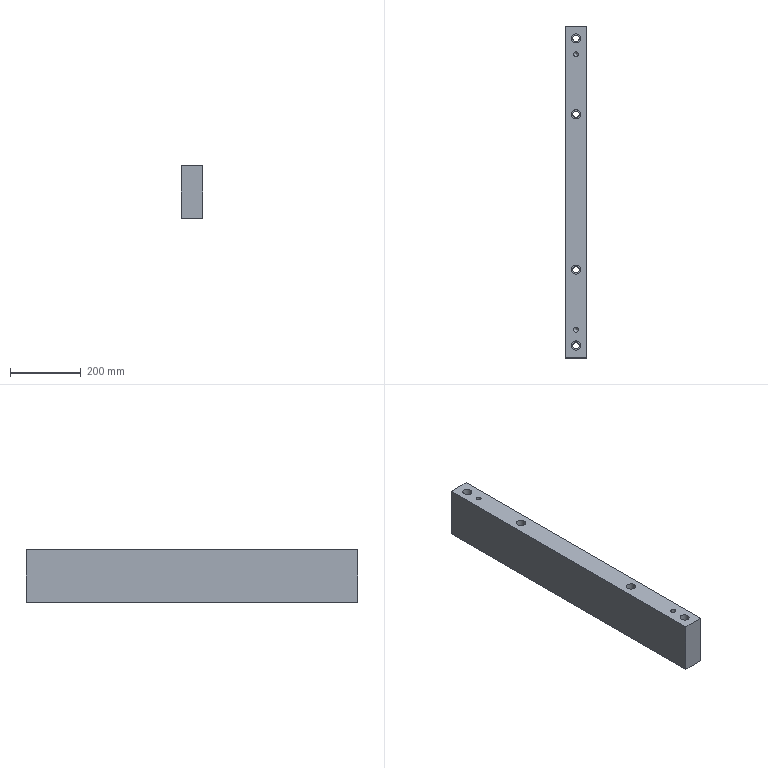Part | STEP file | lll_id1778_x_t | 1 solid | 22 faces | box 60 x 940 x 147.5 mm | volume 8080772 mm3 | plane 10 | cylinder 10 | cone 2 | commonest cylinder face diameters 18.009 x4 26.008 x4 14.506 x2
STEP:
#1=CARTESIAN_POINT('',(3486.439,220.,370.));
#2=VERTEX_POINT('',#1);
#3=CARTESIAN_POINT('',(3473.435,220.,370.));
#4=DIRECTION('',(0.,0.,1.));
#5=DIRECTION('',(1.,0.,0.));
#6=AXIS2_PLACEMENT_3D('',#3,#4,#5);
#7=CIRCLE('',#6,13.004);
#8=EDGE_CURVE('',#2,#2,#7,.T.);
#9=ORIENTED_EDGE('',*,*,#8,.F.);
#10=EDGE_LOOP('',(#9));
#11=FACE_BOUND('',#10,.T.);
#12=CARTESIAN_POINT('',(3486.439,-220.,370.));
#13=VERTEX_POINT('',#12);
#14=CARTESIAN_POINT('',(3473.435,-220.,370.));
#15=DIRECTION('',(0.,0.,-1.));
#16=DIRECTION('',(1.,0.,0.));
#17=AXIS2_PLACEMENT_3D('',#14,#15,#16);
#18=CIRCLE('',#17,13.004);
#19=EDGE_CURVE('',#13,#13,#18,.T.);
#20=ORIENTED_EDGE('',*,*,#19,.T.);
#21=EDGE_LOOP('',(#20));
#22=FACE_BOUND('',#21,.T.);
#23=CARTESIAN_POINT('',(3486.439,-435.,370.));
#24=VERTEX_POINT('',#23);
#25=CARTESIAN_POINT('',(3473.435,-435.,370.));
#26=DIRECTION('',(0.,0.,-1.));
#27=DIRECTION('',(1.,0.,0.));
#28=AXIS2_PLACEMENT_3D('',#25,#26,#27);
#29=CIRCLE('',#28,13.004);
#30=EDGE_CURVE('',#24,#24,#29,.T.);
#31=ORIENTED_EDGE('',*,*,#30,.T.);
#32=EDGE_LOOP('',(#31));
#33=FACE_BOUND('',#32,.T.);
#34=CARTESIAN_POINT('',(3503.435,470.,370.));
#35=VERTEX_POINT('',#34);
#36=CARTESIAN_POINT('',(3443.435,470.,370.));
#37=VERTEX_POINT('',#36);
#38=CARTESIAN_POINT('',(7413.435,470.,370.));
#39=DIRECTION('',(-1.,0.,0.));
#40=VECTOR('',#39,1.);
#41=LINE('',#38,#40);
#42=EDGE_CURVE('',#35,#37,#41,.T.);
#43=ORIENTED_EDGE('',*,*,#42,.T.);
#44=CARTESIAN_POINT('',(3443.435,-470.,370.));
#45=VERTEX_POINT('',#44);
#46=CARTESIAN_POINT('',(3443.435,600.,370.));
#47=DIRECTION('',(0.,-1.,0.));
#48=VECTOR('',#47,1.);
#49=LINE('',#46,#48);
#50=EDGE_CURVE('',#37,#45,#49,.T.);
#51=ORIENTED_EDGE('',*,*,#50,.T.);
#52=CARTESIAN_POINT('',(3503.435,-470.,370.));
#53=VERTEX_POINT('',#52);
#54=CARTESIAN_POINT('',(3443.435,-470.,370.));
#55=DIRECTION('',(1.,0.,0.));
#56=VECTOR('',#55,1.);
#57=LINE('',#54,#56);
#58=EDGE_CURVE('',#45,#53,#57,.T.);
#59=ORIENTED_EDGE('',*,*,#58,.T.);
#60=CARTESIAN_POINT('',(3503.435,1.,370.));
#61=DIRECTION('',(0.,1.,0.));
#62=VECTOR('',#61,1.);
#63=LINE('',#60,#62);
#64=EDGE_CURVE('',#53,#35,#63,.T.);
#65=ORIENTED_EDGE('',*,*,#64,.T.);
#66=EDGE_LOOP('',(#43,#51,#59,#65));
#67=FACE_BOUND('',#66,.T.);
#68=CARTESIAN_POINT('',(3486.439,435.,370.));
#69=VERTEX_POINT('',#68);
#70=CARTESIAN_POINT('',(3473.435,435.,370.));
#71=DIRECTION('',(0.,0.,1.));
#72=DIRECTION('',(1.,0.,0.));
#73=AXIS2_PLACEMENT_3D('',#70,#71,#72);
#74=CIRCLE('',#73,13.004);
#75=EDGE_CURVE('',#69,#69,#74,.T.);
#76=ORIENTED_EDGE('',*,*,#75,.F.);
#77=EDGE_LOOP('',(#76));
#78=FACE_BOUND('',#77,.T.);
#79=CARTESIAN_POINT('',(3480.688,-390.,370.));
#80=VERTEX_POINT('',#79);
#81=CARTESIAN_POINT('',(3473.435,-390.,370.));
#82=DIRECTION('',(0.,0.,-1.));
#83=DIRECTION('',(1.,0.,0.));
#84=AXIS2_PLACEMENT_3D('',#81,#82,#83);
#85=CIRCLE('',#84,7.253);
#86=EDGE_CURVE('',#80,#80,#85,.T.);
#87=ORIENTED_EDGE('',*,*,#86,.T.);
#88=EDGE_LOOP('',(#87));
#89=FACE_BOUND('',#88,.T.);
#90=CARTESIAN_POINT('',(3480.688,390.,370.));
#91=VERTEX_POINT('',#90);
#92=CARTESIAN_POINT('',(3473.435,390.,370.));
#93=DIRECTION('',(0.,0.,1.));
#94=DIRECTION('',(1.,0.,0.));
#95=AXIS2_PLACEMENT_3D('',#92,#93,#94);
#96=CIRCLE('',#95,7.253);
#97=EDGE_CURVE('',#91,#91,#96,.T.);
#98=ORIENTED_EDGE('',*,*,#97,.F.);
#99=EDGE_LOOP('',(#98));
#100=FACE_BOUND('',#99,.T.);
#101=CARTESIAN_POINT('',(1257.12,1.,370.));
#102=DIRECTION('',(0.,0.,-1.));
#103=DIRECTION('',(1.,0.,0.));
#104=AXIS2_PLACEMENT_3D('',#101,#102,#103);
#105=PLANE('',#104);
#106=ADVANCED_FACE('',(#11,#22,#33,#67,#78,#89,#100),#105,.F.);
#107=CARTESIAN_POINT('',(3482.44,435.,222.5));
#108=VERTEX_POINT('',#107);
#109=CARTESIAN_POINT('',(3473.435,435.,222.5));
#110=DIRECTION('',(0.,0.,-1.));
#111=DIRECTION('',(1.,0.,0.));
#112=AXIS2_PLACEMENT_3D('',#109,#110,#111);
#113=CIRCLE('',#112,9.005);
#114=EDGE_CURVE('',#108,#108,#113,.T.);
#115=ORIENTED_EDGE('',*,*,#114,.F.);
#116=EDGE_LOOP('',(#115));
#117=FACE_BOUND('',#116,.T.);
#118=CARTESIAN_POINT('',(3482.44,220.,222.5));
#119=VERTEX_POINT('',#118);
#120=CARTESIAN_POINT('',(3473.435,220.,222.5));
#121=DIRECTION('',(0.,0.,-1.));
#122=DIRECTION('',(1.,0.,0.));
#123=AXIS2_PLACEMENT_3D('',#120,#121,#122);
#124=CIRCLE('',#123,9.005);
#125=EDGE_CURVE('',#119,#119,#124,.T.);
#126=ORIENTED_EDGE('',*,*,#125,.F.);
#127=EDGE_LOOP('',(#126));
#128=FACE_BOUND('',#127,.T.);
#129=CARTESIAN_POINT('',(3482.44,-435.,222.5));
#130=VERTEX_POINT('',#129);
#131=CARTESIAN_POINT('',(3473.435,-435.,222.5));
#132=DIRECTION('',(0.,0.,1.));
#133=DIRECTION('',(1.,0.,0.));
#134=AXIS2_PLACEMENT_3D('',#131,#132,#133);
#135=CIRCLE('',#134,9.005);
#136=EDGE_CURVE('',#130,#130,#135,.T.);
#137=ORIENTED_EDGE('',*,*,#136,.T.);
#138=EDGE_LOOP('',(#137));
#139=FACE_BOUND('',#138,.T.);
#140=CARTESIAN_POINT('',(3503.435,470.,222.5));
#141=VERTEX_POINT('',#140);
#142=CARTESIAN_POINT('',(3503.435,-470.,222.5));
#143=VERTEX_POINT('',#142);
#144=CARTESIAN_POINT('',(3503.435,1.,222.5));
#145=DIRECTION('',(0.,-1.,0.));
#146=VECTOR('',#145,1.);
#147=LINE('',#144,#146);
#148=EDGE_CURVE('',#141,#143,#147,.T.);
#149=ORIENTED_EDGE('',*,*,#148,.T.);
#150=CARTESIAN_POINT('',(3443.435,-470.,222.5));
#151=VERTEX_POINT('',#150);
#152=CARTESIAN_POINT('',(3443.435,-470.,222.5));
#153=DIRECTION('',(1.,0.,0.));
#154=VECTOR('',#153,1.);
#155=LINE('',#152,#154);
#156=EDGE_CURVE('',#151,#143,#155,.T.);
#157=ORIENTED_EDGE('',*,*,#156,.F.);
#158=CARTESIAN_POINT('',(3443.435,470.,222.5));
#159=VERTEX_POINT('',#158);
#160=CARTESIAN_POINT('',(3443.435,600.,222.5));
#161=DIRECTION('',(0.,-1.,0.));
#162=VECTOR('',#161,1.);
#163=LINE('',#160,#162);
#164=EDGE_CURVE('',#159,#151,#163,.T.);
#165=ORIENTED_EDGE('',*,*,#164,.F.);
#166=CARTESIAN_POINT('',(7413.435,470.,222.5));
#167=DIRECTION('',(-1.,0.,0.));
#168=VECTOR('',#167,1.);
#169=LINE('',#166,#168);
#170=EDGE_CURVE('',#141,#159,#169,.T.);
#171=ORIENTED_EDGE('',*,*,#170,.F.);
#172=EDGE_LOOP('',(#149,#157,#165,#171));
#173=FACE_BOUND('',#172,.T.);
#174=CARTESIAN_POINT('',(3482.44,-220.,222.5));
#175=VERTEX_POINT('',#174);
#176=CARTESIAN_POINT('',(3473.435,-220.,222.5));
#177=DIRECTION('',(0.,0.,1.));
#178=DIRECTION('',(1.,0.,0.));
#179=AXIS2_PLACEMENT_3D('',#176,#177,#178);
#180=CIRCLE('',#179,9.005);
#181=EDGE_CURVE('',#175,#175,#180,.T.);
#182=ORIENTED_EDGE('',*,*,#181,.T.);
#183=EDGE_LOOP('',(#182));
#184=FACE_BOUND('',#183,.T.);
#185=CARTESIAN_POINT('',(1257.12,1.,222.5));
#186=DIRECTION('',(0.,0.,-1.));
#187=DIRECTION('',(1.,0.,0.));
#188=AXIS2_PLACEMENT_3D('',#185,#186,#187);
#189=PLANE('',#188);
#190=ADVANCED_FACE('',(#117,#128,#139,#173,#184),#189,.T.);
#191=ORIENTED_EDGE('',*,*,#164,.T.);
#192=CARTESIAN_POINT('',(3443.435,-470.,360.));
#193=DIRECTION('',(0.,0.,-1.));
#194=VECTOR('',#193,1.);
#195=LINE('',#192,#194);
#196=EDGE_CURVE('',#45,#151,#195,.T.);
#197=ORIENTED_EDGE('',*,*,#196,.F.);
#198=ORIENTED_EDGE('',*,*,#50,.F.);
#199=CARTESIAN_POINT('',(3443.435,470.,360.));
#200=DIRECTION('',(0.,0.,-1.));
#201=VECTOR('',#200,1.);
#202=LINE('',#199,#201);
#203=EDGE_CURVE('',#37,#159,#202,.T.);
#204=ORIENTED_EDGE('',*,*,#203,.T.);
#205=EDGE_LOOP('',(#191,#197,#198,#204));
#206=FACE_OUTER_BOUND('',#205,.T.);
#207=CARTESIAN_POINT('',(3443.435,600.,360.));
#208=DIRECTION('',(-1.,0.,0.));
#209=DIRECTION('',(0.,0.,-1.));
#210=AXIS2_PLACEMENT_3D('',#207,#208,#209);
#211=PLANE('',#210);
#212=ADVANCED_FACE('',(#206),#211,.T.);
#213=CARTESIAN_POINT('',(3503.435,-470.,360.));
#214=DIRECTION('',(0.,0.,-1.));
#215=VECTOR('',#214,1.);
#216=LINE('',#213,#215);
#217=EDGE_CURVE('',#53,#143,#216,.T.);
#218=ORIENTED_EDGE('',*,*,#217,.F.);
#219=ORIENTED_EDGE('',*,*,#58,.F.);
#220=ORIENTED_EDGE('',*,*,#196,.T.);
#221=ORIENTED_EDGE('',*,*,#156,.T.);
#222=EDGE_LOOP('',(#218,#219,#220,#221));
#223=FACE_OUTER_BOUND('',#222,.T.);
#224=CARTESIAN_POINT('',(3443.435,-470.,360.));
#225=DIRECTION('',(0.,-1.,0.));
#226=DIRECTION('',(0.,0.,-1.));
#227=AXIS2_PLACEMENT_3D('',#224,#225,#226);
#228=PLANE('',#227);
#229=ADVANCED_FACE('',(#223),#228,.T.);
#230=CARTESIAN_POINT('',(3503.435,470.,360.));
#231=DIRECTION('',(0.,0.,1.));
#232=VECTOR('',#231,1.);
#233=LINE('',#230,#232);
#234=EDGE_CURVE('',#141,#35,#233,.T.);
#235=ORIENTED_EDGE('',*,*,#234,.F.);
#236=ORIENTED_EDGE('',*,*,#170,.T.);
#237=ORIENTED_EDGE('',*,*,#203,.F.);
#238=ORIENTED_EDGE('',*,*,#42,.F.);
#239=EDGE_LOOP('',(#235,#236,#237,#238));
#240=FACE_OUTER_BOUND('',#239,.T.);
#241=CARTESIAN_POINT('',(7413.435,470.,360.));
#242=DIRECTION('',(0.,1.,0.));
#243=DIRECTION('',(0.,0.,1.));
#244=AXIS2_PLACEMENT_3D('',#241,#242,#243);
#245=PLANE('',#244);
#246=ADVANCED_FACE('',(#240),#245,.T.);
#247=ORIENTED_EDGE('',*,*,#234,.T.);
#248=ORIENTED_EDGE('',*,*,#64,.F.);
#249=ORIENTED_EDGE('',*,*,#217,.T.);
#250=ORIENTED_EDGE('',*,*,#148,.F.);
#251=EDGE_LOOP('',(#247,#248,#249,#250));
#252=FACE_OUTER_BOUND('',#251,.T.);
#253=CARTESIAN_POINT('',(3503.435,0.,291.25));
#254=DIRECTION('',(-1.,0.,0.));
#255=DIRECTION('',(0.,0.,-1.));
#256=AXIS2_PLACEMENT_3D('',#253,#254,#255);
#257=PLANE('',#256);
#258=ADVANCED_FACE('',(#252),#257,.F.);
#259=CARTESIAN_POINT('',(3464.431,-435.,302.5));
#260=VERTEX_POINT('',#259);
#261=CARTESIAN_POINT('',(3473.435,-435.,302.5));
#262=DIRECTION('',(0.,0.,-1.));
#263=DIRECTION('',(-1.,0.,0.));
#264=AXIS2_PLACEMENT_3D('',#261,#262,#263);
#265=CIRCLE('',#264,9.005);
#266=EDGE_CURVE('',#260,#260,#265,.T.);
#267=ORIENTED_EDGE('',*,*,#266,.F.);
#268=EDGE_LOOP('',(#267));
#269=FACE_BOUND('',#268,.T.);
#270=ORIENTED_EDGE('',*,*,#136,.F.);
#271=EDGE_LOOP('',(#270));
#272=FACE_BOUND('',#271,.T.);
#273=CARTESIAN_POINT('',(3473.435,-435.,420.));
#274=DIRECTION('',(0.,0.,-1.));
#275=DIRECTION('',(1.,0.,0.));
#276=AXIS2_PLACEMENT_3D('',#273,#274,#275);
#277=CYLINDRICAL_SURFACE('',#276,9.005);
#278=ADVANCED_FACE('',(#269,#272),#277,.F.);
#279=ORIENTED_EDGE('',*,*,#266,.T.);
#280=EDGE_LOOP('',(#279));
#281=FACE_BOUND('',#280,.T.);
#282=CARTESIAN_POINT('',(3486.439,-435.,302.5));
#283=VERTEX_POINT('',#282);
#284=CARTESIAN_POINT('',(3473.435,-435.,302.5));
#285=DIRECTION('',(0.,0.,-1.));
#286=DIRECTION('',(-1.,0.,0.));
#287=AXIS2_PLACEMENT_3D('',#284,#285,#286);
#288=CIRCLE('',#287,13.004);
#289=EDGE_CURVE('',#283,#283,#288,.T.);
#290=ORIENTED_EDGE('',*,*,#289,.F.);
#291=EDGE_LOOP('',(#290));
#292=FACE_BOUND('',#291,.T.);
#293=CARTESIAN_POINT('',(3473.435,-435.,302.5));
#294=DIRECTION('',(0.,0.,-1.));
#295=DIRECTION('',(-1.,0.,0.));
#296=AXIS2_PLACEMENT_3D('',#293,#294,#295);
#297=PLANE('',#296);
#298=ADVANCED_FACE('',(#281,#292),#297,.F.);
#299=ORIENTED_EDGE('',*,*,#289,.T.);
#300=EDGE_LOOP('',(#299));
#301=FACE_BOUND('',#300,.T.);
#302=ORIENTED_EDGE('',*,*,#30,.F.);
#303=EDGE_LOOP('',(#302));
#304=FACE_BOUND('',#303,.T.);
#305=CARTESIAN_POINT('',(3473.435,-435.,420.));
#306=DIRECTION('',(0.,0.,-1.));
#307=DIRECTION('',(1.,0.,0.));
#308=AXIS2_PLACEMENT_3D('',#305,#306,#307);
#309=CYLINDRICAL_SURFACE('',#308,13.004);
#310=ADVANCED_FACE('',(#301,#304),#309,.F.);
#311=CARTESIAN_POINT('',(3464.431,-220.,302.5));
#312=VERTEX_POINT('',#311);
#313=CARTESIAN_POINT('',(3473.435,-220.,302.5));
#314=DIRECTION('',(0.,0.,-1.));
#315=DIRECTION('',(-1.,0.,0.));
#316=AXIS2_PLACEMENT_3D('',#313,#314,#315);
#317=CIRCLE('',#316,9.005);
#318=EDGE_CURVE('',#312,#312,#317,.T.);
#319=ORIENTED_EDGE('',*,*,#318,.F.);
#320=EDGE_LOOP('',(#319));
#321=FACE_BOUND('',#320,.T.);
#322=ORIENTED_EDGE('',*,*,#181,.F.);
#323=EDGE_LOOP('',(#322));
#324=FACE_BOUND('',#323,.T.);
#325=CARTESIAN_POINT('',(3473.435,-220.,420.));
#326=DIRECTION('',(0.,0.,-1.));
#327=DIRECTION('',(1.,0.,0.));
#328=AXIS2_PLACEMENT_3D('',#325,#326,#327);
#329=CYLINDRICAL_SURFACE('',#328,9.005);
#330=ADVANCED_FACE('',(#321,#324),#329,.F.);
#331=ORIENTED_EDGE('',*,*,#318,.T.);
#332=EDGE_LOOP('',(#331));
#333=FACE_BOUND('',#332,.T.);
#334=CARTESIAN_POINT('',(3486.439,-220.,302.5));
#335=VERTEX_POINT('',#334);
#336=CARTESIAN_POINT('',(3473.435,-220.,302.5));
#337=DIRECTION('',(0.,0.,-1.));
#338=DIRECTION('',(1.,0.,0.));
#339=AXIS2_PLACEMENT_3D('',#336,#337,#338);
#340=CIRCLE('',#339,13.004);
#341=EDGE_CURVE('',#335,#335,#340,.T.);
#342=ORIENTED_EDGE('',*,*,#341,.F.);
#343=EDGE_LOOP('',(#342));
#344=FACE_BOUND('',#343,.T.);
#345=CARTESIAN_POINT('',(3473.435,-220.,302.5));
#346=DIRECTION('',(0.,0.,-1.));
#347=DIRECTION('',(-1.,0.,0.));
#348=AXIS2_PLACEMENT_3D('',#345,#346,#347);
#349=PLANE('',#348);
#350=ADVANCED_FACE('',(#333,#344),#349,.F.);
#351=ORIENTED_EDGE('',*,*,#341,.T.);
#352=EDGE_LOOP('',(#351));
#353=FACE_BOUND('',#352,.T.);
#354=ORIENTED_EDGE('',*,*,#19,.F.);
#355=EDGE_LOOP('',(#354));
#356=FACE_BOUND('',#355,.T.);
#357=CARTESIAN_POINT('',(3473.435,-220.,420.));
#358=DIRECTION('',(0.,0.,-1.));
#359=DIRECTION('',(1.,0.,0.));
#360=AXIS2_PLACEMENT_3D('',#357,#358,#359);
#361=CYLINDRICAL_SURFACE('',#360,13.004);
#362=ADVANCED_FACE('',(#353,#356),#361,.F.);
#363=CARTESIAN_POINT('',(3464.431,220.,302.5));
#364=VERTEX_POINT('',#363);
#365=CARTESIAN_POINT('',(3473.435,220.,302.5));
#366=DIRECTION('',(0.,0.,1.));
#367=DIRECTION('',(-1.,0.,0.));
#368=AXIS2_PLACEMENT_3D('',#365,#366,#367);
#369=CIRCLE('',#368,9.005);
#370=EDGE_CURVE('',#364,#364,#369,.T.);
#371=ORIENTED_EDGE('',*,*,#370,.T.);
#372=EDGE_LOOP('',(#371));
#373=FACE_BOUND('',#372,.T.);
#374=ORIENTED_EDGE('',*,*,#125,.T.);
#375=EDGE_LOOP('',(#374));
#376=FACE_BOUND('',#375,.T.);
#377=CARTESIAN_POINT('',(3473.435,220.,420.));
#378=DIRECTION('',(0.,0.,-1.));
#379=DIRECTION('',(1.,0.,0.));
#380=AXIS2_PLACEMENT_3D('',#377,#378,#379);
#381=CYLINDRICAL_SURFACE('',#380,9.005);
#382=ADVANCED_FACE('',(#373,#376),#381,.F.);
#383=ORIENTED_EDGE('',*,*,#370,.F.);
#384=EDGE_LOOP('',(#383));
#385=FACE_BOUND('',#384,.T.);
#386=CARTESIAN_POINT('',(3486.439,220.,302.5));
#387=VERTEX_POINT('',#386);
#388=CARTESIAN_POINT('',(3473.435,220.,302.5));
#389=DIRECTION('',(0.,0.,1.));
#390=DIRECTION('',(1.,0.,0.));
#391=AXIS2_PLACEMENT_3D('',#388,#389,#390);
#392=CIRCLE('',#391,13.004);
#393=EDGE_CURVE('',#387,#387,#392,.T.);
#394=ORIENTED_EDGE('',*,*,#393,.T.);
#395=EDGE_LOOP('',(#394));
#396=FACE_BOUND('',#395,.T.);
#397=CARTESIAN_POINT('',(3473.435,220.,302.5));
#398=DIRECTION('',(0.,0.,-1.));
#399=DIRECTION('',(-1.,0.,0.));
#400=AXIS2_PLACEMENT_3D('',#397,#398,#399);
#401=PLANE('',#400);
#402=ADVANCED_FACE('',(#385,#396),#401,.F.);
#403=ORIENTED_EDGE('',*,*,#393,.F.);
#404=EDGE_LOOP('',(#403));
#405=FACE_BOUND('',#404,.T.);
#406=ORIENTED_EDGE('',*,*,#8,.T.);
#407=EDGE_LOOP('',(#406));
#408=FACE_BOUND('',#407,.T.);
#409=CARTESIAN_POINT('',(3473.435,220.,420.));
#410=DIRECTION('',(0.,0.,-1.));
#411=DIRECTION('',(1.,0.,0.));
#412=AXIS2_PLACEMENT_3D('',#409,#410,#411);
#413=CYLINDRICAL_SURFACE('',#412,13.004);
#414=ADVANCED_FACE('',(#405,#408),#413,.F.);
#415=CARTESIAN_POINT('',(3464.431,435.,302.5));
#416=VERTEX_POINT('',#415);
#417=CARTESIAN_POINT('',(3473.435,435.,302.5));
#418=DIRECTION('',(0.,0.,1.));
#419=DIRECTION('',(-1.,0.,0.));
#420=AXIS2_PLACEMENT_3D('',#417,#418,#419);
#421=CIRCLE('',#420,9.005);
#422=EDGE_CURVE('',#416,#416,#421,.T.);
#423=ORIENTED_EDGE('',*,*,#422,.T.);
#424=EDGE_LOOP('',(#423));
#425=FACE_BOUND('',#424,.T.);
#426=ORIENTED_EDGE('',*,*,#114,.T.);
#427=EDGE_LOOP('',(#426));
#428=FACE_BOUND('',#427,.T.);
#429=CARTESIAN_POINT('',(3473.435,435.,420.));
#430=DIRECTION('',(0.,0.,-1.));
#431=DIRECTION('',(1.,0.,0.));
#432=AXIS2_PLACEMENT_3D('',#429,#430,#431);
#433=CYLINDRICAL_SURFACE('',#432,9.005);
#434=ADVANCED_FACE('',(#425,#428),#433,.F.);
#435=ORIENTED_EDGE('',*,*,#422,.F.);
#436=EDGE_LOOP('',(#435));
#437=FACE_BOUND('',#436,.T.);
#438=CARTESIAN_POINT('',(3486.439,435.,302.5));
#439=VERTEX_POINT('',#438);
#440=CARTESIAN_POINT('',(3473.435,435.,302.5));
#441=DIRECTION('',(0.,0.,1.));
#442=DIRECTION('',(1.,0.,0.));
#443=AXIS2_PLACEMENT_3D('',#440,#441,#442);
#444=CIRCLE('',#443,13.004);
#445=EDGE_CURVE('',#439,#439,#444,.T.);
#446=ORIENTED_EDGE('',*,*,#445,.T.);
#447=EDGE_LOOP('',(#446));
#448=FACE_BOUND('',#447,.T.);
#449=CARTESIAN_POINT('',(3473.435,435.,302.5));
#450=DIRECTION('',(0.,0.,-1.));
#451=DIRECTION('',(-1.,0.,0.));
#452=AXIS2_PLACEMENT_3D('',#449,#450,#451);
#453=PLANE('',#452);
#454=ADVANCED_FACE('',(#437,#448),#453,.F.);
#455=ORIENTED_EDGE('',*,*,#445,.F.);
#456=EDGE_LOOP('',(#455));
#457=FACE_BOUND('',#456,.T.);
#458=ORIENTED_EDGE('',*,*,#75,.T.);
#459=EDGE_LOOP('',(#458));
#460=FACE_BOUND('',#459,.T.);
#461=CARTESIAN_POINT('',(3473.435,435.,420.));
#462=DIRECTION('',(0.,0.,-1.));
#463=DIRECTION('',(1.,0.,0.));
#464=AXIS2_PLACEMENT_3D('',#461,#462,#463);
#465=CYLINDRICAL_SURFACE('',#464,13.004);
#466=ADVANCED_FACE('',(#457,#460),#465,.F.);
#467=CARTESIAN_POINT('',(3466.182,-390.,332.247));
#468=VERTEX_POINT('',#467);
#469=CARTESIAN_POINT('',(3473.435,-390.,332.247));
#470=DIRECTION('',(0.,0.,-1.));
#471=DIRECTION('',(-1.,0.,0.));
#472=AXIS2_PLACEMENT_3D('',#469,#470,#471);
#473=CIRCLE('',#472,7.253);
#474=EDGE_CURVE('',#468,#468,#473,.T.);
#475=ORIENTED_EDGE('',*,*,#474,.T.);
#476=EDGE_LOOP('',(#475));
#477=FACE_BOUND('',#476,.T.);
#478=ORIENTED_EDGE('',*,*,#86,.F.);
#479=EDGE_LOOP('',(#478));
#480=FACE_BOUND('',#479,.T.);
#481=CARTESIAN_POINT('',(3473.435,-390.,370.));
#482=DIRECTION('',(0.,0.,-1.));
#483=DIRECTION('',(1.,0.,0.));
#484=AXIS2_PLACEMENT_3D('',#481,#482,#483);
#485=CYLINDRICAL_SURFACE('',#484,7.253);
#486=ADVANCED_FACE('',(#477,#480),#485,.F.);
#487=CARTESIAN_POINT('',(3473.435,-390.,324.994));
#488=VERTEX_POINT('',#487);
#489=VERTEX_LOOP('',#488);
#490=FACE_BOUND('',#489,.T.);
#491=ORIENTED_EDGE('',*,*,#474,.F.);
#492=EDGE_LOOP('',(#491));
#493=FACE_BOUND('',#492,.T.);
#494=CARTESIAN_POINT('',(3473.435,-390.,332.247));
#495=DIRECTION('',(0.,0.,1.));
#496=DIRECTION('',(1.,0.,0.));
#497=AXIS2_PLACEMENT_3D('',#494,#495,#496);
#498=CONICAL_SURFACE('',#497,7.253,45.);
#499=ADVANCED_FACE('',(#490,#493),#498,.F.);
#500=CARTESIAN_POINT('',(3466.182,390.,332.247));
#501=VERTEX_POINT('',#500);
#502=CARTESIAN_POINT('',(3473.435,390.,332.247));
#503=DIRECTION('',(0.,0.,1.));
#504=DIRECTION('',(-1.,0.,0.));
#505=AXIS2_PLACEMENT_3D('',#502,#503,#504);
#506=CIRCLE('',#505,7.253);
#507=EDGE_CURVE('',#501,#501,#506,.T.);
#508=ORIENTED_EDGE('',*,*,#507,.F.);
#509=EDGE_LOOP('',(#508));
#510=FACE_BOUND('',#509,.T.);
#511=ORIENTED_EDGE('',*,*,#97,.T.);
#512=EDGE_LOOP('',(#511));
#513=FACE_BOUND('',#512,.T.);
#514=CARTESIAN_POINT('',(3473.435,390.,370.));
#515=DIRECTION('',(0.,0.,-1.));
#516=DIRECTION('',(1.,0.,0.));
#517=AXIS2_PLACEMENT_3D('',#514,#515,#516);
#518=CYLINDRICAL_SURFACE('',#517,7.253);
#519=ADVANCED_FACE('',(#510,#513),#518,.F.);
#520=CARTESIAN_POINT('',(3473.435,390.,324.994));
#521=VERTEX_POINT('',#520);
#522=VERTEX_LOOP('',#521);
#523=FACE_BOUND('',#522,.T.);
#524=ORIENTED_EDGE('',*,*,#507,.T.);
#525=EDGE_LOOP('',(#524));
#526=FACE_BOUND('',#525,.T.);
#527=CARTESIAN_POINT('',(3473.435,390.,332.247));
#528=DIRECTION('',(0.,0.,1.));
#529=DIRECTION('',(1.,0.,0.));
#530=AXIS2_PLACEMENT_3D('',#527,#528,#529);
#531=CONICAL_SURFACE('',#530,7.253,45.);
#532=ADVANCED_FACE('',(#523,#526),#531,.F.);
#533=CLOSED_SHELL('',(#106,#190,#212,#229,#246,#258,#278,#298,#310,#330,#350,#362,#382,#402,#414,#434,#454,#466,#486,#499,#519,#532));
#534=MANIFOLD_SOLID_BREP('',#533);
#535=(LENGTH_UNIT()NAMED_UNIT(*)SI_UNIT(.MILLI.,.METRE.));
#536=UNCERTAINTY_MEASURE_WITH_UNIT(LENGTH_MEASURE(0.00002),#535,'','');
#537=(NAMED_UNIT(*)PLANE_ANGLE_UNIT()SI_UNIT($,.RADIAN.));
#538=PLANE_ANGLE_MEASURE_WITH_UNIT(PLANE_ANGLE_MEASURE(0.01745),#537);
#539=DIMENSIONAL_EXPONENTS(0.,0.,0.,0.,0.,0.,0.);
#540=(CONVERSION_BASED_UNIT('DEGREE',#538)NAMED_UNIT(#539)PLANE_ANGLE_UNIT());
#541=(NAMED_UNIT(*)SI_UNIT($,.STERADIAN.)SOLID_ANGLE_UNIT());
#542=(GEOMETRIC_REPRESENTATION_CONTEXT(3)GLOBAL_UNCERTAINTY_ASSIGNED_CONTEXT((#536))GLOBAL_UNIT_ASSIGNED_CONTEXT((#535,#540,#541))REPRESENTATION_CONTEXT('',''));
#543=ADVANCED_BREP_SHAPE_REPRESENTATION('',(#534),#542);